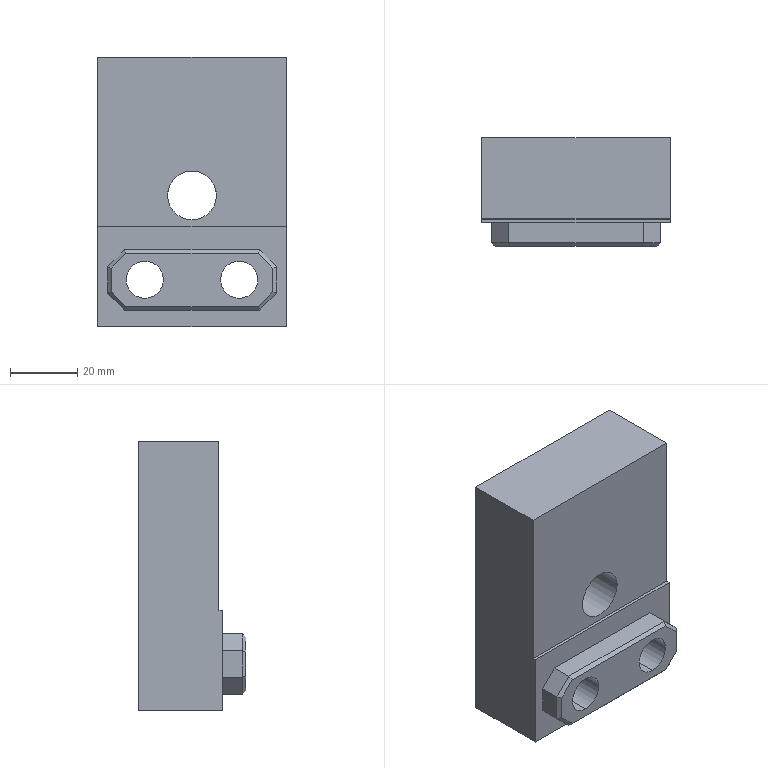Part | Creo | 1 solid | 53 faces | box 56 x 32 x 80 mm | volume 99961 mm3 | plane 27 | cylinder 18 | cone 8 | commonest cylinder face diameters 6.71 x4 8 x4 11 x4 18 x4 14.5 x2
STEP:
#1=CARTESIAN_POINT('',(0.,0.,0.));
#2=DIRECTION('',(0.,0.,1.));
#3=DIRECTION('',(1.,0.,0.));
#4=AXIS2_PLACEMENT_3D('',#1,#2,#3);
#5=CARTESIAN_POINT('',(-28.05,250.,-50.133));
#6=VERTEX_POINT('',#5);
#7=CARTESIAN_POINT('',(-28.05,250.,-20.267));
#8=VERTEX_POINT('',#7);
#9=CARTESIAN_POINT('',(-28.05,250.,-50.133));
#10=DIRECTION('',(0.,0.,1.));
#11=VECTOR('',#10,29.866);
#12=LINE('',#9,#11);
#13=EDGE_CURVE('',#6,#8,#12,.T.);
#14=ORIENTED_EDGE('',*,*,#13,.T.);
#15=CARTESIAN_POINT('',(27.95,250.,-20.267));
#16=VERTEX_POINT('',#15);
#17=CARTESIAN_POINT('',(27.95,250.,-20.267));
#18=DIRECTION('',(-1.,0.,0.));
#19=VECTOR('',#18,56.);
#20=LINE('',#17,#19);
#21=EDGE_CURVE('',#16,#8,#20,.T.);
#22=ORIENTED_EDGE('',*,*,#21,.F.);
#23=CARTESIAN_POINT('',(27.95,250.,-50.133));
#24=VERTEX_POINT('',#23);
#25=CARTESIAN_POINT('',(27.95,250.,-20.267));
#26=DIRECTION('',(0.,0.,-1.));
#27=VECTOR('',#26,29.866);
#28=LINE('',#25,#27);
#29=EDGE_CURVE('',#16,#24,#28,.T.);
#30=ORIENTED_EDGE('',*,*,#29,.T.);
#31=CARTESIAN_POINT('',(27.95,250.,-50.133));
#32=DIRECTION('',(-1.,0.,0.));
#33=VECTOR('',#32,56.);
#34=LINE('',#31,#33);
#35=EDGE_CURVE('',#24,#6,#34,.T.);
#36=ORIENTED_EDGE('',*,*,#35,.T.);
#37=EDGE_LOOP('',(#14,#22,#30,#36));
#38=FACE_OUTER_BOUND('',#37,.F.);
#39=CARTESIAN_POINT('',(-25.05,250.,-40.133));
#40=VERTEX_POINT('',#39);
#41=CARTESIAN_POINT('',(-25.05,250.,-32.267));
#42=VERTEX_POINT('',#41);
#43=CARTESIAN_POINT('',(-25.05,250.,-40.133));
#44=DIRECTION('',(0.,0.,1.));
#45=VECTOR('',#44,7.867);
#46=LINE('',#43,#45);
#47=EDGE_CURVE('',#40,#42,#46,.T.);
#48=ORIENTED_EDGE('',*,*,#47,.F.);
#49=CARTESIAN_POINT('',(-20.05,250.,-45.133));
#50=VERTEX_POINT('',#49);
#51=CARTESIAN_POINT('',(-20.05,250.,-45.133));
#52=DIRECTION('',(-0.7071,0.,0.7071));
#53=VECTOR('',#52,7.071);
#54=LINE('',#51,#53);
#55=EDGE_CURVE('',#50,#40,#54,.T.);
#56=ORIENTED_EDGE('',*,*,#55,.F.);
#57=CARTESIAN_POINT('',(19.95,250.,-45.133));
#58=VERTEX_POINT('',#57);
#59=CARTESIAN_POINT('',(-20.05,250.,-45.133));
#60=DIRECTION('',(1.,0.,0.));
#61=VECTOR('',#60,40.);
#62=LINE('',#59,#61);
#63=EDGE_CURVE('',#50,#58,#62,.T.);
#64=ORIENTED_EDGE('',*,*,#63,.T.);
#65=CARTESIAN_POINT('',(24.95,250.,-40.133));
#66=VERTEX_POINT('',#65);
#67=CARTESIAN_POINT('',(24.95,250.,-40.133));
#68=DIRECTION('',(-0.7071,0.,-0.7071));
#69=VECTOR('',#68,7.071);
#70=LINE('',#67,#69);
#71=EDGE_CURVE('',#66,#58,#70,.T.);
#72=ORIENTED_EDGE('',*,*,#71,.F.);
#73=CARTESIAN_POINT('',(24.95,250.,-32.267));
#74=VERTEX_POINT('',#73);
#75=CARTESIAN_POINT('',(24.95,250.,-32.267));
#76=DIRECTION('',(0.,0.,-1.));
#77=VECTOR('',#76,7.867);
#78=LINE('',#75,#77);
#79=EDGE_CURVE('',#74,#66,#78,.T.);
#80=ORIENTED_EDGE('',*,*,#79,.F.);
#81=CARTESIAN_POINT('',(19.95,250.,-27.267));
#82=VERTEX_POINT('',#81);
#83=CARTESIAN_POINT('',(19.95,250.,-27.267));
#84=DIRECTION('',(0.7071,0.,-0.7071));
#85=VECTOR('',#84,7.071);
#86=LINE('',#83,#85);
#87=EDGE_CURVE('',#82,#74,#86,.T.);
#88=ORIENTED_EDGE('',*,*,#87,.F.);
#89=CARTESIAN_POINT('',(-20.05,250.,-27.267));
#90=VERTEX_POINT('',#89);
#91=CARTESIAN_POINT('',(19.95,250.,-27.267));
#92=DIRECTION('',(-1.,0.,0.));
#93=VECTOR('',#92,40.);
#94=LINE('',#91,#93);
#95=EDGE_CURVE('',#82,#90,#94,.T.);
#96=ORIENTED_EDGE('',*,*,#95,.T.);
#97=CARTESIAN_POINT('',(-25.05,250.,-32.267));
#98=DIRECTION('',(0.7071,0.,0.7071));
#99=VECTOR('',#98,7.071);
#100=LINE('',#97,#99);
#101=EDGE_CURVE('',#42,#90,#100,.T.);
#102=ORIENTED_EDGE('',*,*,#101,.F.);
#103=EDGE_LOOP('',(#48,#56,#64,#72,#80,#88,#96,#102));
#104=FACE_BOUND('',#103,.F.);
#105=CARTESIAN_POINT('',(0.,250.,0.));
#106=DIRECTION('',(0.,-1.,0.));
#107=DIRECTION('',(0.,0.,-1.));
#108=AXIS2_PLACEMENT_3D('',#105,#106,#107);
#109=PLANE('',#108);
#110=ADVANCED_FACE('',(#38,#104),#109,.T.);
#111=CARTESIAN_POINT('',(-28.05,275.,-50.133));
#112=VERTEX_POINT('',#111);
#113=CARTESIAN_POINT('',(-28.05,275.,-50.133));
#114=DIRECTION('',(0.,-1.,0.));
#115=VECTOR('',#114,25.);
#116=LINE('',#113,#115);
#117=EDGE_CURVE('',#112,#6,#116,.T.);
#118=ORIENTED_EDGE('',*,*,#117,.F.);
#119=CARTESIAN_POINT('',(-28.05,275.,29.866));
#120=VERTEX_POINT('',#119);
#121=CARTESIAN_POINT('',(-28.05,275.,-50.133));
#122=DIRECTION('',(0.,0.,1.));
#123=VECTOR('',#122,80.);
#124=LINE('',#121,#123);
#125=EDGE_CURVE('',#112,#120,#124,.T.);
#126=ORIENTED_EDGE('',*,*,#125,.T.);
#127=CARTESIAN_POINT('',(-28.05,251.,29.866));
#128=VERTEX_POINT('',#127);
#129=CARTESIAN_POINT('',(-28.05,275.,29.866));
#130=DIRECTION('',(0.,-1.,0.));
#131=VECTOR('',#130,24.);
#132=LINE('',#129,#131);
#133=EDGE_CURVE('',#120,#128,#132,.T.);
#134=ORIENTED_EDGE('',*,*,#133,.T.);
#135=CARTESIAN_POINT('',(-28.05,251.,-20.267));
#136=VERTEX_POINT('',#135);
#137=CARTESIAN_POINT('',(-28.05,251.,-20.267));
#138=DIRECTION('',(0.,0.,1.));
#139=VECTOR('',#138,50.133);
#140=LINE('',#137,#139);
#141=EDGE_CURVE('',#136,#128,#140,.T.);
#142=ORIENTED_EDGE('',*,*,#141,.F.);
#143=CARTESIAN_POINT('',(-28.05,250.,-20.267));
#144=DIRECTION('',(0.,1.,0.));
#145=VECTOR('',#144,1.);
#146=LINE('',#143,#145);
#147=EDGE_CURVE('',#8,#136,#146,.T.);
#148=ORIENTED_EDGE('',*,*,#147,.F.);
#149=ORIENTED_EDGE('',*,*,#13,.F.);
#150=EDGE_LOOP('',(#118,#126,#134,#142,#148,#149));
#151=FACE_OUTER_BOUND('',#150,.F.);
#152=CARTESIAN_POINT('',(-28.05,250.,4.867));
#153=DIRECTION('',(1.,0.,0.));
#154=DIRECTION('',(0.,0.,-1.));
#155=AXIS2_PLACEMENT_3D('',#152,#153,#154);
#156=PLANE('',#155);
#157=ADVANCED_FACE('',(#151),#156,.F.);
#158=CARTESIAN_POINT('',(27.95,275.,-50.133));
#159=VERTEX_POINT('',#158);
#160=CARTESIAN_POINT('',(27.95,275.,-50.133));
#161=DIRECTION('',(-1.,0.,0.));
#162=VECTOR('',#161,56.);
#163=LINE('',#160,#162);
#164=EDGE_CURVE('',#159,#112,#163,.T.);
#165=ORIENTED_EDGE('',*,*,#164,.T.);
#166=ORIENTED_EDGE('',*,*,#117,.T.);
#167=ORIENTED_EDGE('',*,*,#35,.F.);
#168=CARTESIAN_POINT('',(27.95,275.,-50.133));
#169=DIRECTION('',(0.,-1.,0.));
#170=VECTOR('',#169,25.);
#171=LINE('',#168,#170);
#172=EDGE_CURVE('',#159,#24,#171,.T.);
#173=ORIENTED_EDGE('',*,*,#172,.F.);
#174=EDGE_LOOP('',(#165,#166,#167,#173));
#175=FACE_OUTER_BOUND('',#174,.F.);
#176=CARTESIAN_POINT('',(-25.05,250.,-50.133));
#177=DIRECTION('',(0.,0.,1.));
#178=DIRECTION('',(1.,0.,0.));
#179=AXIS2_PLACEMENT_3D('',#176,#177,#178);
#180=PLANE('',#179);
#181=ADVANCED_FACE('',(#175),#180,.F.);
#182=CARTESIAN_POINT('',(27.95,275.,29.866));
#183=VERTEX_POINT('',#182);
#184=CARTESIAN_POINT('',(27.95,275.,29.866));
#185=DIRECTION('',(0.,0.,-1.));
#186=VECTOR('',#185,80.);
#187=LINE('',#184,#186);
#188=EDGE_CURVE('',#183,#159,#187,.T.);
#189=ORIENTED_EDGE('',*,*,#188,.F.);
#190=CARTESIAN_POINT('',(-28.05,275.,29.866));
#191=DIRECTION('',(1.,0.,0.));
#192=VECTOR('',#191,56.);
#193=LINE('',#190,#192);
#194=EDGE_CURVE('',#120,#183,#193,.T.);
#195=ORIENTED_EDGE('',*,*,#194,.F.);
#196=ORIENTED_EDGE('',*,*,#125,.F.);
#197=ORIENTED_EDGE('',*,*,#164,.F.);
#198=EDGE_LOOP('',(#189,#195,#196,#197));
#199=FACE_OUTER_BOUND('',#198,.F.);
#200=CARTESIAN_POINT('',(-0.05,275.,-18.384));
#201=VERTEX_POINT('',#200);
#202=CARTESIAN_POINT('',(7.2,275.,-11.133));
#203=VERTEX_POINT('',#202);
#204=CARTESIAN_POINT('',(-0.05,275.,-11.133));
#205=DIRECTION('',(0.,-1.,0.));
#206=DIRECTION('',(0.,0.,-1.));
#207=AXIS2_PLACEMENT_3D('',#204,#205,#206);
#208=CIRCLE('',#207,7.25);
#209=EDGE_CURVE('',#201,#203,#208,.T.);
#210=ORIENTED_EDGE('',*,*,#209,.F.);
#211=CARTESIAN_POINT('',(-7.3,275.,-11.133));
#212=VERTEX_POINT('',#211);
#213=CARTESIAN_POINT('',(-0.05,275.,-11.133));
#214=DIRECTION('',(0.,-1.,0.));
#215=DIRECTION('',(-1.,0.,0.));
#216=AXIS2_PLACEMENT_3D('',#213,#214,#215);
#217=CIRCLE('',#216,7.25);
#218=EDGE_CURVE('',#212,#201,#217,.T.);
#219=ORIENTED_EDGE('',*,*,#218,.F.);
#220=CARTESIAN_POINT('',(-0.05,275.,-3.884));
#221=VERTEX_POINT('',#220);
#222=CARTESIAN_POINT('',(-0.05,275.,-11.133));
#223=DIRECTION('',(0.,-1.,0.));
#224=DIRECTION('',(0.,0.,1.));
#225=AXIS2_PLACEMENT_3D('',#222,#223,#224);
#226=CIRCLE('',#225,7.25);
#227=EDGE_CURVE('',#221,#212,#226,.T.);
#228=ORIENTED_EDGE('',*,*,#227,.F.);
#229=CARTESIAN_POINT('',(-0.05,275.,-11.133));
#230=DIRECTION('',(0.,-1.,0.));
#231=DIRECTION('',(1.,0.,0.));
#232=AXIS2_PLACEMENT_3D('',#229,#230,#231);
#233=CIRCLE('',#232,7.25);
#234=EDGE_CURVE('',#203,#221,#233,.T.);
#235=ORIENTED_EDGE('',*,*,#234,.F.);
#236=EDGE_LOOP('',(#210,#219,#228,#235));
#237=FACE_BOUND('',#236,.F.);
#238=CARTESIAN_POINT('',(13.95,275.,-45.133));
#239=VERTEX_POINT('',#238);
#240=CARTESIAN_POINT('',(13.95,275.,-27.134));
#241=VERTEX_POINT('',#240);
#242=CARTESIAN_POINT('',(13.95,275.,-36.133));
#243=DIRECTION('',(0.,-1.,0.));
#244=DIRECTION('',(0.,0.,-1.));
#245=AXIS2_PLACEMENT_3D('',#242,#243,#244);
#246=CIRCLE('',#245,9.);
#247=EDGE_CURVE('',#239,#241,#246,.T.);
#248=ORIENTED_EDGE('',*,*,#247,.F.);
#249=CARTESIAN_POINT('',(13.95,275.,-36.133));
#250=DIRECTION('',(0.,-1.,0.));
#251=DIRECTION('',(0.,0.,1.));
#252=AXIS2_PLACEMENT_3D('',#249,#250,#251);
#253=CIRCLE('',#252,9.);
#254=EDGE_CURVE('',#241,#239,#253,.T.);
#255=ORIENTED_EDGE('',*,*,#254,.F.);
#256=EDGE_LOOP('',(#248,#255));
#257=FACE_BOUND('',#256,.F.);
#258=CARTESIAN_POINT('',(-14.05,275.,-45.133));
#259=VERTEX_POINT('',#258);
#260=CARTESIAN_POINT('',(-14.05,275.,-27.134));
#261=VERTEX_POINT('',#260);
#262=CARTESIAN_POINT('',(-14.05,275.,-36.133));
#263=DIRECTION('',(0.,-1.,0.));
#264=DIRECTION('',(0.,0.,-1.));
#265=AXIS2_PLACEMENT_3D('',#262,#263,#264);
#266=CIRCLE('',#265,9.);
#267=EDGE_CURVE('',#259,#261,#266,.T.);
#268=ORIENTED_EDGE('',*,*,#267,.F.);
#269=CARTESIAN_POINT('',(-14.05,275.,-36.133));
#270=DIRECTION('',(0.,-1.,0.));
#271=DIRECTION('',(0.,0.,1.));
#272=AXIS2_PLACEMENT_3D('',#269,#270,#271);
#273=CIRCLE('',#272,9.);
#274=EDGE_CURVE('',#261,#259,#273,.T.);
#275=ORIENTED_EDGE('',*,*,#274,.F.);
#276=EDGE_LOOP('',(#268,#275));
#277=FACE_BOUND('',#276,.F.);
#278=CARTESIAN_POINT('',(15.95,275.,18.42));
#279=VERTEX_POINT('',#278);
#280=CARTESIAN_POINT('',(7.95,275.,18.42));
#281=VERTEX_POINT('',#280);
#282=CARTESIAN_POINT('',(11.95,275.,18.42));
#283=DIRECTION('',(0.,-1.,0.));
#284=DIRECTION('',(1.,0.,0.));
#285=AXIS2_PLACEMENT_3D('',#282,#283,#284);
#286=CIRCLE('',#285,4.);
#287=EDGE_CURVE('',#279,#281,#286,.T.);
#288=ORIENTED_EDGE('',*,*,#287,.F.);
#289=CARTESIAN_POINT('',(11.95,275.,18.42));
#290=DIRECTION('',(0.,-1.,0.));
#291=DIRECTION('',(-1.,0.,0.));
#292=AXIS2_PLACEMENT_3D('',#289,#290,#291);
#293=CIRCLE('',#292,4.);
#294=EDGE_CURVE('',#281,#279,#293,.T.);
#295=ORIENTED_EDGE('',*,*,#294,.F.);
#296=EDGE_LOOP('',(#288,#295));
#297=FACE_BOUND('',#296,.F.);
#298=CARTESIAN_POINT('',(-8.05,275.,18.42));
#299=VERTEX_POINT('',#298);
#300=CARTESIAN_POINT('',(-16.05,275.,18.42));
#301=VERTEX_POINT('',#300);
#302=CARTESIAN_POINT('',(-12.05,275.,18.42));
#303=DIRECTION('',(0.,-1.,0.));
#304=DIRECTION('',(1.,0.,0.));
#305=AXIS2_PLACEMENT_3D('',#302,#303,#304);
#306=CIRCLE('',#305,4.);
#307=EDGE_CURVE('',#299,#301,#306,.T.);
#308=ORIENTED_EDGE('',*,*,#307,.F.);
#309=CARTESIAN_POINT('',(-12.05,275.,18.42));
#310=DIRECTION('',(0.,-1.,0.));
#311=DIRECTION('',(-1.,0.,0.));
#312=AXIS2_PLACEMENT_3D('',#309,#310,#311);
#313=CIRCLE('',#312,4.);
#314=EDGE_CURVE('',#301,#299,#313,.T.);
#315=ORIENTED_EDGE('',*,*,#314,.F.);
#316=EDGE_LOOP('',(#308,#315));
#317=FACE_BOUND('',#316,.F.);
#318=CARTESIAN_POINT('',(0.,275.,0.));
#319=DIRECTION('',(0.,-1.,0.));
#320=DIRECTION('',(0.,0.,-1.));
#321=AXIS2_PLACEMENT_3D('',#318,#319,#320);
#322=PLANE('',#321);
#323=ADVANCED_FACE('',(#199,#237,#257,#277,#297,#317),#322,.F.);
#324=CARTESIAN_POINT('',(7.2,251.,-11.133));
#325=VERTEX_POINT('',#324);
#326=CARTESIAN_POINT('',(-0.05,251.,-18.384));
#327=VERTEX_POINT('',#326);
#328=CARTESIAN_POINT('',(-0.05,251.,-11.133));
#329=DIRECTION('',(0.,1.,0.));
#330=DIRECTION('',(1.,0.,0.));
#331=AXIS2_PLACEMENT_3D('',#328,#329,#330);
#332=CIRCLE('',#331,7.25);
#333=EDGE_CURVE('',#325,#327,#332,.T.);
#334=ORIENTED_EDGE('',*,*,#333,.T.);
#335=CARTESIAN_POINT('',(-7.3,251.,-11.133));
#336=VERTEX_POINT('',#335);
#337=CARTESIAN_POINT('',(-0.05,251.,-11.133));
#338=DIRECTION('',(0.,1.,0.));
#339=DIRECTION('',(0.,0.,-1.));
#340=AXIS2_PLACEMENT_3D('',#337,#338,#339);
#341=CIRCLE('',#340,7.25);
#342=EDGE_CURVE('',#327,#336,#341,.T.);
#343=ORIENTED_EDGE('',*,*,#342,.T.);
#344=CARTESIAN_POINT('',(-7.3,251.,-11.133));
#345=DIRECTION('',(0.,1.,0.));
#346=VECTOR('',#345,24.);
#347=LINE('',#344,#346);
#348=EDGE_CURVE('',#336,#212,#347,.T.);
#349=ORIENTED_EDGE('',*,*,#348,.T.);
#350=ORIENTED_EDGE('',*,*,#218,.T.);
#351=ORIENTED_EDGE('',*,*,#209,.T.);
#352=CARTESIAN_POINT('',(7.2,251.,-11.133));
#353=DIRECTION('',(0.,1.,0.));
#354=VECTOR('',#353,24.);
#355=LINE('',#352,#354);
#356=EDGE_CURVE('',#325,#203,#355,.T.);
#357=ORIENTED_EDGE('',*,*,#356,.F.);
#358=EDGE_LOOP('',(#334,#343,#349,#350,#351,#357));
#359=FACE_OUTER_BOUND('',#358,.F.);
#360=CARTESIAN_POINT('',(-0.05,205.,-11.133));
#361=DIRECTION('',(0.,1.,0.));
#362=DIRECTION('',(-1.,0.,0.));
#363=AXIS2_PLACEMENT_3D('',#360,#361,#362);
#364=CYLINDRICAL_SURFACE('',#363,7.25);
#365=ADVANCED_FACE('',(#359),#364,.F.);
#366=ORIENTED_EDGE('',*,*,#141,.T.);
#367=CARTESIAN_POINT('',(27.95,251.,29.866));
#368=VERTEX_POINT('',#367);
#369=CARTESIAN_POINT('',(-28.05,251.,29.866));
#370=DIRECTION('',(1.,0.,0.));
#371=VECTOR('',#370,56.);
#372=LINE('',#369,#371);
#373=EDGE_CURVE('',#128,#368,#372,.T.);
#374=ORIENTED_EDGE('',*,*,#373,.T.);
#375=CARTESIAN_POINT('',(27.95,251.,-20.267));
#376=VERTEX_POINT('',#375);
#377=CARTESIAN_POINT('',(27.95,251.,29.866));
#378=DIRECTION('',(0.,0.,-1.));
#379=VECTOR('',#378,50.133);
#380=LINE('',#377,#379);
#381=EDGE_CURVE('',#368,#376,#380,.T.);
#382=ORIENTED_EDGE('',*,*,#381,.T.);
#383=CARTESIAN_POINT('',(-28.05,251.,-20.267));
#384=DIRECTION('',(1.,0.,0.));
#385=VECTOR('',#384,56.);
#386=LINE('',#383,#385);
#387=EDGE_CURVE('',#136,#376,#386,.T.);
#388=ORIENTED_EDGE('',*,*,#387,.F.);
#389=EDGE_LOOP('',(#366,#374,#382,#388));
#390=FACE_OUTER_BOUND('',#389,.F.);
#391=ORIENTED_EDGE('',*,*,#342,.F.);
#392=ORIENTED_EDGE('',*,*,#333,.F.);
#393=CARTESIAN_POINT('',(-0.05,251.,-11.133));
#394=DIRECTION('',(0.,1.,0.));
#395=DIRECTION('',(-1.,0.,0.));
#396=AXIS2_PLACEMENT_3D('',#393,#394,#395);
#397=CIRCLE('',#396,7.25);
#398=EDGE_CURVE('',#336,#325,#397,.T.);
#399=ORIENTED_EDGE('',*,*,#398,.F.);
#400=EDGE_LOOP('',(#391,#392,#399));
#401=FACE_BOUND('',#400,.F.);
#402=CARTESIAN_POINT('',(0.,251.,0.));
#403=DIRECTION('',(0.,-1.,0.));
#404=DIRECTION('',(0.,0.,-1.));
#405=AXIS2_PLACEMENT_3D('',#402,#403,#404);
#406=PLANE('',#405);
#407=ADVANCED_FACE('',(#390,#401),#406,.T.);
#408=ORIENTED_EDGE('',*,*,#398,.T.);
#409=ORIENTED_EDGE('',*,*,#356,.T.);
#410=ORIENTED_EDGE('',*,*,#234,.T.);
#411=ORIENTED_EDGE('',*,*,#227,.T.);
#412=ORIENTED_EDGE('',*,*,#348,.F.);
#413=EDGE_LOOP('',(#408,#409,#410,#411,#412));
#414=FACE_OUTER_BOUND('',#413,.F.);
#415=CARTESIAN_POINT('',(-0.05,205.,-11.133));
#416=DIRECTION('',(0.,1.,0.));
#417=DIRECTION('',(-1.,0.,0.));
#418=AXIS2_PLACEMENT_3D('',#415,#416,#417);
#419=CYLINDRICAL_SURFACE('',#418,7.25);
#420=ADVANCED_FACE('',(#414),#419,.F.);
#421=ORIENTED_EDGE('',*,*,#194,.T.);
#422=CARTESIAN_POINT('',(27.95,275.,29.866));
#423=DIRECTION('',(0.,-1.,0.));
#424=VECTOR('',#423,24.);
#425=LINE('',#422,#424);
#426=EDGE_CURVE('',#183,#368,#425,.T.);
#427=ORIENTED_EDGE('',*,*,#426,.T.);
#428=ORIENTED_EDGE('',*,*,#373,.F.);
#429=ORIENTED_EDGE('',*,*,#133,.F.);
#430=EDGE_LOOP('',(#421,#427,#428,#429));
#431=FACE_OUTER_BOUND('',#430,.F.);
#432=CARTESIAN_POINT('',(24.95,250.,29.866));
#433=DIRECTION('',(0.,0.,-1.));
#434=DIRECTION('',(-1.,0.,0.));
#435=AXIS2_PLACEMENT_3D('',#432,#433,#434);
#436=PLANE('',#435);
#437=ADVANCED_FACE('',(#431),#436,.F.);
#438=ORIENTED_EDGE('',*,*,#29,.F.);
#439=CARTESIAN_POINT('',(27.95,251.,-20.267));
#440=DIRECTION('',(0.,-1.,0.));
#441=VECTOR('',#440,1.);
#442=LINE('',#439,#441);
#443=EDGE_CURVE('',#376,#16,#442,.T.);
#444=ORIENTED_EDGE('',*,*,#443,.F.);
#445=ORIENTED_EDGE('',*,*,#381,.F.);
#446=ORIENTED_EDGE('',*,*,#426,.F.);
#447=ORIENTED_EDGE('',*,*,#188,.T.);
#448=ORIENTED_EDGE('',*,*,#172,.T.);
#449=EDGE_LOOP('',(#438,#444,#445,#446,#447,#448));
#450=FACE_OUTER_BOUND('',#449,.F.);
#451=CARTESIAN_POINT('',(27.95,250.,-50.133));
#452=DIRECTION('',(-1.,0.,0.));
#453=DIRECTION('',(0.,0.,1.));
#454=AXIS2_PLACEMENT_3D('',#451,#452,#453);
#455=PLANE('',#454);
#456=ADVANCED_FACE('',(#450),#455,.F.);
#457=ORIENTED_EDGE('',*,*,#443,.T.);
#458=ORIENTED_EDGE('',*,*,#21,.T.);
#459=ORIENTED_EDGE('',*,*,#147,.T.);
#460=ORIENTED_EDGE('',*,*,#387,.T.);
#461=EDGE_LOOP('',(#457,#458,#459,#460));
#462=FACE_OUTER_BOUND('',#461,.F.);
#463=CARTESIAN_POINT('',(-0.05,205.5,-20.267));
#464=DIRECTION('',(0.,0.,-1.));
#465=DIRECTION('',(-1.,0.,0.));
#466=AXIS2_PLACEMENT_3D('',#463,#464,#465);
#467=PLANE('',#466);
#468=ADVANCED_FACE('',(#462),#467,.F.);
#469=CARTESIAN_POINT('',(13.95,264.,-27.134));
#470=VERTEX_POINT('',#469);
#471=CARTESIAN_POINT('',(13.95,264.,-45.133));
#472=VERTEX_POINT('',#471);
#473=CARTESIAN_POINT('',(13.95,264.,-36.133));
#474=DIRECTION('',(0.,1.,0.));
#475=DIRECTION('',(0.,0.,1.));
#476=AXIS2_PLACEMENT_3D('',#473,#474,#475);
#477=CIRCLE('',#476,9.);
#478=EDGE_CURVE('',#470,#472,#477,.T.);
#479=ORIENTED_EDGE('',*,*,#478,.T.);
#480=CARTESIAN_POINT('',(13.95,275.,-45.133));
#481=DIRECTION('',(0.,-1.,0.));
#482=VECTOR('',#481,11.);
#483=LINE('',#480,#482);
#484=EDGE_CURVE('',#239,#472,#483,.T.);
#485=ORIENTED_EDGE('',*,*,#484,.F.);
#486=ORIENTED_EDGE('',*,*,#247,.T.);
#487=CARTESIAN_POINT('',(13.95,275.,-27.134));
#488=DIRECTION('',(0.,-1.,0.));
#489=VECTOR('',#488,11.);
#490=LINE('',#487,#489);
#491=EDGE_CURVE('',#241,#470,#490,.T.);
#492=ORIENTED_EDGE('',*,*,#491,.T.);
#493=EDGE_LOOP('',(#479,#485,#486,#492));
#494=FACE_OUTER_BOUND('',#493,.F.);
#495=CARTESIAN_POINT('',(13.95,275.,-36.133));
#496=DIRECTION('',(0.,-1.,0.));
#497=DIRECTION('',(0.,0.,-1.));
#498=AXIS2_PLACEMENT_3D('',#495,#496,#497);
#499=CYLINDRICAL_SURFACE('',#498,9.);
#500=ADVANCED_FACE('',(#494),#499,.F.);
#501=CARTESIAN_POINT('',(13.95,264.,-36.133));
#502=DIRECTION('',(0.,1.,0.));
#503=DIRECTION('',(0.,0.,-1.));
#504=AXIS2_PLACEMENT_3D('',#501,#502,#503);
#505=CIRCLE('',#504,9.);
#506=EDGE_CURVE('',#472,#470,#505,.T.);
#507=ORIENTED_EDGE('',*,*,#506,.F.);
#508=ORIENTED_EDGE('',*,*,#478,.F.);
#509=EDGE_LOOP('',(#507,#508));
#510=FACE_OUTER_BOUND('',#509,.F.);
#511=CARTESIAN_POINT('',(13.95,264.,-41.633));
#512=VERTEX_POINT('',#511);
#513=CARTESIAN_POINT('',(13.95,264.,-30.634));
#514=VERTEX_POINT('',#513);
#515=CARTESIAN_POINT('',(13.95,264.,-36.133));
#516=DIRECTION('',(0.,-1.,0.));
#517=DIRECTION('',(0.,0.,-1.));
#518=AXIS2_PLACEMENT_3D('',#515,#516,#517);
#519=CIRCLE('',#518,5.5);
#520=EDGE_CURVE('',#512,#514,#519,.T.);
#521=ORIENTED_EDGE('',*,*,#520,.F.);
#522=CARTESIAN_POINT('',(13.95,264.,-36.133));
#523=DIRECTION('',(0.,-1.,0.));
#524=DIRECTION('',(0.,0.,1.));
#525=AXIS2_PLACEMENT_3D('',#522,#523,#524);
#526=CIRCLE('',#525,5.5);
#527=EDGE_CURVE('',#514,#512,#526,.T.);
#528=ORIENTED_EDGE('',*,*,#527,.F.);
#529=EDGE_LOOP('',(#521,#528));
#530=FACE_BOUND('',#529,.F.);
#531=CARTESIAN_POINT('',(13.95,264.,-36.133));
#532=DIRECTION('',(0.,-1.,0.));
#533=DIRECTION('',(0.,0.,-1.));
#534=AXIS2_PLACEMENT_3D('',#531,#532,#533);
#535=PLANE('',#534);
#536=ADVANCED_FACE('',(#510,#530),#535,.F.);
#537=ORIENTED_EDGE('',*,*,#520,.T.);
#538=CARTESIAN_POINT('',(13.95,243.,-30.634));
#539=VERTEX_POINT('',#538);
#540=CARTESIAN_POINT('',(13.95,264.,-30.634));
#541=DIRECTION('',(0.,-1.,0.));
#542=VECTOR('',#541,21.);
#543=LINE('',#540,#542);
#544=EDGE_CURVE('',#514,#539,#543,.T.);
#545=ORIENTED_EDGE('',*,*,#544,.T.);
#546=CARTESIAN_POINT('',(13.95,243.,-41.633));
#547=VERTEX_POINT('',#546);
#548=CARTESIAN_POINT('',(13.95,243.,-36.133));
#549=DIRECTION('',(0.,1.,0.));
#550=DIRECTION('',(0.,0.,1.));
#551=AXIS2_PLACEMENT_3D('',#548,#549,#550);
#552=CIRCLE('',#551,5.5);
#553=EDGE_CURVE('',#539,#547,#552,.T.);
#554=ORIENTED_EDGE('',*,*,#553,.T.);
#555=CARTESIAN_POINT('',(13.95,264.,-41.633));
#556=DIRECTION('',(0.,-1.,0.));
#557=VECTOR('',#556,21.);
#558=LINE('',#555,#557);
#559=EDGE_CURVE('',#512,#547,#558,.T.);
#560=ORIENTED_EDGE('',*,*,#559,.F.);
#561=EDGE_LOOP('',(#537,#545,#554,#560));
#562=FACE_OUTER_BOUND('',#561,.F.);
#563=CARTESIAN_POINT('',(13.95,75.,-36.133));
#564=DIRECTION('',(0.,-1.,0.));
#565=DIRECTION('',(0.,0.,-1.));
#566=AXIS2_PLACEMENT_3D('',#563,#564,#565);
#567=CYLINDRICAL_SURFACE('',#566,5.5);
#568=ADVANCED_FACE('',(#562),#567,.F.);
#569=ORIENTED_EDGE('',*,*,#527,.T.);
#570=ORIENTED_EDGE('',*,*,#559,.T.);
#571=CARTESIAN_POINT('',(13.95,243.,-36.133));
#572=DIRECTION('',(0.,1.,0.));
#573=DIRECTION('',(0.,0.,-1.));
#574=AXIS2_PLACEMENT_3D('',#571,#572,#573);
#575=CIRCLE('',#574,5.5);
#576=EDGE_CURVE('',#547,#539,#575,.T.);
#577=ORIENTED_EDGE('',*,*,#576,.T.);
#578=ORIENTED_EDGE('',*,*,#544,.F.);
#579=EDGE_LOOP('',(#569,#570,#577,#578));
#580=FACE_OUTER_BOUND('',#579,.F.);
#581=CARTESIAN_POINT('',(13.95,75.,-36.133));
#582=DIRECTION('',(0.,-1.,0.));
#583=DIRECTION('',(0.,0.,-1.));
#584=AXIS2_PLACEMENT_3D('',#581,#582,#583);
#585=CYLINDRICAL_SURFACE('',#584,5.5);
#586=ADVANCED_FACE('',(#580),#585,.F.);
#587=CARTESIAN_POINT('',(23.95,243.,-32.681));
#588=VERTEX_POINT('',#587);
#589=CARTESIAN_POINT('',(23.95,243.,-39.719));
#590=VERTEX_POINT('',#589);
#591=CARTESIAN_POINT('',(23.95,243.,-32.681));
#592=DIRECTION('',(0.,0.,-1.));
#593=VECTOR('',#592,7.038);
#594=LINE('',#591,#593);
#595=EDGE_CURVE('',#588,#590,#594,.T.);
#596=ORIENTED_EDGE('',*,*,#595,.T.);
#597=CARTESIAN_POINT('',(19.536,243.,-44.133));
#598=VERTEX_POINT('',#597);
#599=CARTESIAN_POINT('',(19.536,243.,-44.133));
#600=DIRECTION('',(0.7071,0.,0.7071));
#601=VECTOR('',#600,6.243);
#602=LINE('',#599,#601);
#603=EDGE_CURVE('',#598,#590,#602,.T.);
#604=ORIENTED_EDGE('',*,*,#603,.F.);
#605=CARTESIAN_POINT('',(-19.636,243.,-44.133));
#606=VERTEX_POINT('',#605);
#607=CARTESIAN_POINT('',(19.536,243.,-44.133));
#608=DIRECTION('',(-1.,0.,0.));
#609=VECTOR('',#608,39.172);
#610=LINE('',#607,#609);
#611=EDGE_CURVE('',#598,#606,#610,.T.);
#612=ORIENTED_EDGE('',*,*,#611,.T.);
#613=CARTESIAN_POINT('',(-24.05,243.,-39.719));
#614=VERTEX_POINT('',#613);
#615=CARTESIAN_POINT('',(-24.05,243.,-39.719));
#616=DIRECTION('',(0.7071,0.,-0.7071));
#617=VECTOR('',#616,6.243);
#618=LINE('',#615,#617);
#619=EDGE_CURVE('',#614,#606,#618,.T.);
#620=ORIENTED_EDGE('',*,*,#619,.F.);
#621=CARTESIAN_POINT('',(-24.05,243.,-32.681));
#622=VERTEX_POINT('',#621);
#623=CARTESIAN_POINT('',(-24.05,243.,-39.719));
#624=DIRECTION('',(0.,0.,1.));
#625=VECTOR('',#624,7.038);
#626=LINE('',#623,#625);
#627=EDGE_CURVE('',#614,#622,#626,.T.);
#628=ORIENTED_EDGE('',*,*,#627,.T.);
#629=CARTESIAN_POINT('',(-19.636,243.,-28.267));
#630=VERTEX_POINT('',#629);
#631=CARTESIAN_POINT('',(-19.636,243.,-28.267));
#632=DIRECTION('',(-0.7071,0.,-0.7071));
#633=VECTOR('',#632,6.243);
#634=LINE('',#631,#633);
#635=EDGE_CURVE('',#630,#622,#634,.T.);
#636=ORIENTED_EDGE('',*,*,#635,.F.);
#637=CARTESIAN_POINT('',(19.536,243.,-28.267));
#638=VERTEX_POINT('',#637);
#639=CARTESIAN_POINT('',(-19.636,243.,-28.267));
#640=DIRECTION('',(1.,0.,0.));
#641=VECTOR('',#640,39.172);
#642=LINE('',#639,#641);
#643=EDGE_CURVE('',#630,#638,#642,.T.);
#644=ORIENTED_EDGE('',*,*,#643,.T.);
#645=CARTESIAN_POINT('',(23.95,243.,-32.681));
#646=DIRECTION('',(-0.7071,0.,0.7071));
#647=VECTOR('',#646,6.243);
#648=LINE('',#645,#647);
#649=EDGE_CURVE('',#588,#638,#648,.T.);
#650=ORIENTED_EDGE('',*,*,#649,.F.);
#651=EDGE_LOOP('',(#596,#604,#612,#620,#628,#636,#644,#650));
#652=FACE_OUTER_BOUND('',#651,.F.);
#653=CARTESIAN_POINT('',(-14.05,243.,-41.633));
#654=VERTEX_POINT('',#653);
#655=CARTESIAN_POINT('',(-14.05,243.,-30.634));
#656=VERTEX_POINT('',#655);
#657=CARTESIAN_POINT('',(-14.05,243.,-36.133));
#658=DIRECTION('',(0.,1.,0.));
#659=DIRECTION('',(0.,0.,-1.));
#660=AXIS2_PLACEMENT_3D('',#657,#658,#659);
#661=CIRCLE('',#660,5.5);
#662=EDGE_CURVE('',#654,#656,#661,.T.);
#663=ORIENTED_EDGE('',*,*,#662,.F.);
#664=CARTESIAN_POINT('',(-14.05,243.,-36.133));
#665=DIRECTION('',(0.,1.,0.));
#666=DIRECTION('',(0.,0.,1.));
#667=AXIS2_PLACEMENT_3D('',#664,#665,#666);
#668=CIRCLE('',#667,5.5);
#669=EDGE_CURVE('',#656,#654,#668,.T.);
#670=ORIENTED_EDGE('',*,*,#669,.F.);
#671=EDGE_LOOP('',(#663,#670));
#672=FACE_BOUND('',#671,.F.);
#673=ORIENTED_EDGE('',*,*,#576,.F.);
#674=ORIENTED_EDGE('',*,*,#553,.F.);
#675=EDGE_LOOP('',(#673,#674));
#676=FACE_BOUND('',#675,.F.);
#677=CARTESIAN_POINT('',(-0.05,243.,-51.133));
#678=DIRECTION('',(0.,-1.,0.));
#679=DIRECTION('',(0.,0.,-1.));
#680=AXIS2_PLACEMENT_3D('',#677,#678,#679);
#681=PLANE('',#680);
#682=ADVANCED_FACE('',(#652,#672,#676),#681,.T.);
#683=CARTESIAN_POINT('',(24.95,244.,-40.133));
#684=VERTEX_POINT('',#683);
#685=CARTESIAN_POINT('',(24.95,244.,-40.133));
#686=DIRECTION('',(-0.6786,-0.6786,0.2811));
#687=VECTOR('',#686,1.474);
#688=LINE('',#685,#687);
#689=EDGE_CURVE('',#684,#590,#688,.T.);
#690=ORIENTED_EDGE('',*,*,#689,.T.);
#691=ORIENTED_EDGE('',*,*,#595,.F.);
#692=CARTESIAN_POINT('',(24.95,244.,-32.267));
#693=VERTEX_POINT('',#692);
#694=CARTESIAN_POINT('',(24.95,244.,-32.267));
#695=DIRECTION('',(-0.6786,-0.6786,-0.2811));
#696=VECTOR('',#695,1.474);
#697=LINE('',#694,#696);
#698=EDGE_CURVE('',#693,#588,#697,.T.);
#699=ORIENTED_EDGE('',*,*,#698,.F.);
#700=CARTESIAN_POINT('',(24.95,244.,-40.133));
#701=DIRECTION('',(0.,0.,1.));
#702=VECTOR('',#701,7.867);
#703=LINE('',#700,#702);
#704=EDGE_CURVE('',#684,#693,#703,.T.);
#705=ORIENTED_EDGE('',*,*,#704,.F.);
#706=EDGE_LOOP('',(#690,#691,#699,#705));
#707=FACE_OUTER_BOUND('',#706,.F.);
#708=CARTESIAN_POINT('',(23.95,243.,-51.133));
#709=DIRECTION('',(0.7071,-0.7071,0.));
#710=DIRECTION('',(0.,0.,-1.));
#711=AXIS2_PLACEMENT_3D('',#708,#709,#710);
#712=PLANE('',#711);
#713=ADVANCED_FACE('',(#707),#712,.T.);
#714=CARTESIAN_POINT('',(19.95,244.,-45.133));
#715=VERTEX_POINT('',#714);
#716=CARTESIAN_POINT('',(19.95,244.,-45.133));
#717=DIRECTION('',(-0.2811,-0.6786,0.6786));
#718=VECTOR('',#717,1.474);
#719=LINE('',#716,#718);
#720=EDGE_CURVE('',#715,#598,#719,.T.);
#721=ORIENTED_EDGE('',*,*,#720,.T.);
#722=ORIENTED_EDGE('',*,*,#603,.T.);
#723=ORIENTED_EDGE('',*,*,#689,.F.);
#724=CARTESIAN_POINT('',(19.95,244.,-45.133));
#725=DIRECTION('',(0.7071,0.,0.7071));
#726=VECTOR('',#725,7.071);
#727=LINE('',#724,#726);
#728=EDGE_CURVE('',#715,#684,#727,.T.);
#729=ORIENTED_EDGE('',*,*,#728,.F.);
#730=EDGE_LOOP('',(#721,#722,#723,#729));
#731=FACE_OUTER_BOUND('',#730,.F.);
#732=CARTESIAN_POINT('',(6.243,243.,-57.426));
#733=DIRECTION('',(0.5,-0.7071,-0.5));
#734=DIRECTION('',(-0.7071,0.,-0.7071));
#735=AXIS2_PLACEMENT_3D('',#732,#733,#734);
#736=PLANE('',#735);
#737=ADVANCED_FACE('',(#731),#736,.T.);
#738=CARTESIAN_POINT('',(-20.05,244.,-45.133));
#739=VERTEX_POINT('',#738);
#740=CARTESIAN_POINT('',(-20.05,244.,-45.133));
#741=DIRECTION('',(0.2811,-0.6786,0.6786));
#742=VECTOR('',#741,1.474);
#743=LINE('',#740,#742);
#744=EDGE_CURVE('',#739,#606,#743,.T.);
#745=ORIENTED_EDGE('',*,*,#744,.T.);
#746=ORIENTED_EDGE('',*,*,#611,.F.);
#747=ORIENTED_EDGE('',*,*,#720,.F.);
#748=CARTESIAN_POINT('',(-20.05,244.,-45.133));
#749=DIRECTION('',(1.,0.,0.));
#750=VECTOR('',#749,40.);
#751=LINE('',#748,#750);
#752=EDGE_CURVE('',#739,#715,#751,.T.);
#753=ORIENTED_EDGE('',*,*,#752,.F.);
#754=EDGE_LOOP('',(#745,#746,#747,#753));
#755=FACE_OUTER_BOUND('',#754,.F.);
#756=CARTESIAN_POINT('',(-0.05,243.,-44.133));
#757=DIRECTION('',(0.,-0.7071,-0.7071));
#758=DIRECTION('',(-1.,0.,0.));
#759=AXIS2_PLACEMENT_3D('',#756,#757,#758);
#760=PLANE('',#759);
#761=ADVANCED_FACE('',(#755),#760,.T.);
#762=CARTESIAN_POINT('',(-25.05,244.,-40.133));
#763=VERTEX_POINT('',#762);
#764=CARTESIAN_POINT('',(-24.05,243.,-39.719));
#765=DIRECTION('',(-0.6786,0.6786,-0.2811));
#766=VECTOR('',#765,1.474);
#767=LINE('',#764,#766);
#768=EDGE_CURVE('',#614,#763,#767,.T.);
#769=ORIENTED_EDGE('',*,*,#768,.F.);
#770=ORIENTED_EDGE('',*,*,#619,.T.);
#771=ORIENTED_EDGE('',*,*,#744,.F.);
#772=CARTESIAN_POINT('',(-25.05,244.,-40.133));
#773=DIRECTION('',(0.7071,0.,-0.7071));
#774=VECTOR('',#773,7.071);
#775=LINE('',#772,#774);
#776=EDGE_CURVE('',#763,#739,#775,.T.);
#777=ORIENTED_EDGE('',*,*,#776,.F.);
#778=EDGE_LOOP('',(#769,#770,#771,#777));
#779=FACE_OUTER_BOUND('',#778,.F.);
#780=CARTESIAN_POINT('',(-6.343,243.,-57.426));
#781=DIRECTION('',(-0.5,-0.7071,-0.5));
#782=DIRECTION('',(-0.7071,0.,0.7071));
#783=AXIS2_PLACEMENT_3D('',#780,#781,#782);
#784=PLANE('',#783);
#785=ADVANCED_FACE('',(#779),#784,.T.);
#786=ORIENTED_EDGE('',*,*,#768,.T.);
#787=CARTESIAN_POINT('',(-25.05,244.,-32.267));
#788=VERTEX_POINT('',#787);
#789=CARTESIAN_POINT('',(-25.05,244.,-32.267));
#790=DIRECTION('',(0.,0.,-1.));
#791=VECTOR('',#790,7.867);
#792=LINE('',#789,#791);
#793=EDGE_CURVE('',#788,#763,#792,.T.);
#794=ORIENTED_EDGE('',*,*,#793,.F.);
#795=CARTESIAN_POINT('',(-24.05,243.,-32.681));
#796=DIRECTION('',(-0.6786,0.6786,0.2811));
#797=VECTOR('',#796,1.474);
#798=LINE('',#795,#797);
#799=EDGE_CURVE('',#622,#788,#798,.T.);
#800=ORIENTED_EDGE('',*,*,#799,.F.);
#801=ORIENTED_EDGE('',*,*,#627,.F.);
#802=EDGE_LOOP('',(#786,#794,#800,#801));
#803=FACE_OUTER_BOUND('',#802,.F.);
#804=CARTESIAN_POINT('',(-25.05,244.,4.867));
#805=DIRECTION('',(-0.7071,-0.7071,0.));
#806=DIRECTION('',(0.,0.,-1.));
#807=AXIS2_PLACEMENT_3D('',#804,#805,#806);
#808=PLANE('',#807);
#809=ADVANCED_FACE('',(#803),#808,.T.);
#810=CARTESIAN_POINT('',(-25.05,250.,-32.267));
#811=DIRECTION('',(0.,-1.,0.));
#812=VECTOR('',#811,6.);
#813=LINE('',#810,#812);
#814=EDGE_CURVE('',#42,#788,#813,.T.);
#815=ORIENTED_EDGE('',*,*,#814,.T.);
#816=ORIENTED_EDGE('',*,*,#793,.T.);
#817=CARTESIAN_POINT('',(-25.05,244.,-40.133));
#818=DIRECTION('',(0.,1.,0.));
#819=VECTOR('',#818,6.);
#820=LINE('',#817,#819);
#821=EDGE_CURVE('',#763,#40,#820,.T.);
#822=ORIENTED_EDGE('',*,*,#821,.T.);
#823=ORIENTED_EDGE('',*,*,#47,.T.);
#824=EDGE_LOOP('',(#815,#816,#822,#823));
#825=FACE_OUTER_BOUND('',#824,.F.);
#826=CARTESIAN_POINT('',(-25.05,250.,4.867));
#827=DIRECTION('',(1.,0.,0.));
#828=DIRECTION('',(0.,0.,-1.));
#829=AXIS2_PLACEMENT_3D('',#826,#827,#828);
#830=PLANE('',#829);
#831=ADVANCED_FACE('',(#825),#830,.F.);
#832=ORIENTED_EDGE('',*,*,#814,.F.);
#833=ORIENTED_EDGE('',*,*,#101,.T.);
#834=CARTESIAN_POINT('',(-20.05,244.,-27.267));
#835=VERTEX_POINT('',#834);
#836=CARTESIAN_POINT('',(-20.05,244.,-27.267));
#837=DIRECTION('',(0.,1.,0.));
#838=VECTOR('',#837,6.);
#839=LINE('',#836,#838);
#840=EDGE_CURVE('',#835,#90,#839,.T.);
#841=ORIENTED_EDGE('',*,*,#840,.F.);
#842=CARTESIAN_POINT('',(-20.05,244.,-27.267));
#843=DIRECTION('',(-0.7071,0.,-0.7071));
#844=VECTOR('',#843,7.071);
#845=LINE('',#842,#844);
#846=EDGE_CURVE('',#835,#788,#845,.T.);
#847=ORIENTED_EDGE('',*,*,#846,.T.);
#848=EDGE_LOOP('',(#832,#833,#841,#847));
#849=FACE_OUTER_BOUND('',#848,.F.);
#850=CARTESIAN_POINT('',(-25.05,250.,-32.267));
#851=DIRECTION('',(0.7071,0.,-0.7071));
#852=DIRECTION('',(0.,1.,0.));
#853=AXIS2_PLACEMENT_3D('',#850,#851,#852);
#854=PLANE('',#853);
#855=ADVANCED_FACE('',(#849),#854,.F.);
#856=ORIENTED_EDGE('',*,*,#840,.T.);
#857=ORIENTED_EDGE('',*,*,#95,.F.);
#858=CARTESIAN_POINT('',(19.95,244.,-27.267));
#859=VERTEX_POINT('',#858);
#860=CARTESIAN_POINT('',(19.95,250.,-27.267));
#861=DIRECTION('',(0.,-1.,0.));
#862=VECTOR('',#861,6.);
#863=LINE('',#860,#862);
#864=EDGE_CURVE('',#82,#859,#863,.T.);
#865=ORIENTED_EDGE('',*,*,#864,.T.);
#866=CARTESIAN_POINT('',(19.95,244.,-27.267));
#867=DIRECTION('',(-1.,0.,0.));
#868=VECTOR('',#867,40.);
#869=LINE('',#866,#868);
#870=EDGE_CURVE('',#859,#835,#869,.T.);
#871=ORIENTED_EDGE('',*,*,#870,.T.);
#872=EDGE_LOOP('',(#856,#857,#865,#871));
#873=FACE_OUTER_BOUND('',#872,.F.);
#874=CARTESIAN_POINT('',(-0.05,205.5,-27.267));
#875=DIRECTION('',(0.,0.,-1.));
#876=DIRECTION('',(-1.,0.,0.));
#877=AXIS2_PLACEMENT_3D('',#874,#875,#876);
#878=PLANE('',#877);
#879=ADVANCED_FACE('',(#873),#878,.F.);
#880=ORIENTED_EDGE('',*,*,#864,.F.);
#881=ORIENTED_EDGE('',*,*,#87,.T.);
#882=CARTESIAN_POINT('',(24.95,244.,-32.267));
#883=DIRECTION('',(0.,1.,0.));
#884=VECTOR('',#883,6.);
#885=LINE('',#882,#884);
#886=EDGE_CURVE('',#693,#74,#885,.T.);
#887=ORIENTED_EDGE('',*,*,#886,.F.);
#888=CARTESIAN_POINT('',(24.95,244.,-32.267));
#889=DIRECTION('',(-0.7071,0.,0.7071));
#890=VECTOR('',#889,7.071);
#891=LINE('',#888,#890);
#892=EDGE_CURVE('',#693,#859,#891,.T.);
#893=ORIENTED_EDGE('',*,*,#892,.T.);
#894=EDGE_LOOP('',(#880,#881,#887,#893));
#895=FACE_OUTER_BOUND('',#894,.F.);
#896=CARTESIAN_POINT('',(24.95,250.,-32.267));
#897=DIRECTION('',(-0.7071,0.,-0.7071));
#898=DIRECTION('',(0.,-1.,0.));
#899=AXIS2_PLACEMENT_3D('',#896,#897,#898);
#900=PLANE('',#899);
#901=ADVANCED_FACE('',(#895),#900,.F.);
#902=CARTESIAN_POINT('',(24.95,250.,-40.133));
#903=DIRECTION('',(0.,-1.,0.));
#904=VECTOR('',#903,6.);
#905=LINE('',#902,#904);
#906=EDGE_CURVE('',#66,#684,#905,.T.);
#907=ORIENTED_EDGE('',*,*,#906,.T.);
#908=ORIENTED_EDGE('',*,*,#704,.T.);
#909=ORIENTED_EDGE('',*,*,#886,.T.);
#910=ORIENTED_EDGE('',*,*,#79,.T.);
#911=EDGE_LOOP('',(#907,#908,#909,#910));
#912=FACE_OUTER_BOUND('',#911,.F.);
#913=CARTESIAN_POINT('',(24.95,250.,-50.133));
#914=DIRECTION('',(-1.,0.,0.));
#915=DIRECTION('',(0.,0.,1.));
#916=AXIS2_PLACEMENT_3D('',#913,#914,#915);
#917=PLANE('',#916);
#918=ADVANCED_FACE('',(#912),#917,.F.);
#919=ORIENTED_EDGE('',*,*,#906,.F.);
#920=ORIENTED_EDGE('',*,*,#71,.T.);
#921=CARTESIAN_POINT('',(19.95,244.,-45.133));
#922=DIRECTION('',(0.,1.,0.));
#923=VECTOR('',#922,6.);
#924=LINE('',#921,#923);
#925=EDGE_CURVE('',#715,#58,#924,.T.);
#926=ORIENTED_EDGE('',*,*,#925,.F.);
#927=ORIENTED_EDGE('',*,*,#728,.T.);
#928=EDGE_LOOP('',(#919,#920,#926,#927));
#929=FACE_OUTER_BOUND('',#928,.F.);
#930=CARTESIAN_POINT('',(24.95,250.,-40.133));
#931=DIRECTION('',(-0.7071,0.,0.7071));
#932=DIRECTION('',(0.,1.,0.));
#933=AXIS2_PLACEMENT_3D('',#930,#931,#932);
#934=PLANE('',#933);
#935=ADVANCED_FACE('',(#929),#934,.F.);
#936=ORIENTED_EDGE('',*,*,#925,.T.);
#937=ORIENTED_EDGE('',*,*,#63,.F.);
#938=CARTESIAN_POINT('',(-20.05,250.,-45.133));
#939=DIRECTION('',(0.,-1.,0.));
#940=VECTOR('',#939,6.);
#941=LINE('',#938,#940);
#942=EDGE_CURVE('',#50,#739,#941,.T.);
#943=ORIENTED_EDGE('',*,*,#942,.T.);
#944=ORIENTED_EDGE('',*,*,#752,.T.);
#945=EDGE_LOOP('',(#936,#937,#943,#944));
#946=FACE_OUTER_BOUND('',#945,.F.);
#947=CARTESIAN_POINT('',(-25.05,250.,-45.133));
#948=DIRECTION('',(0.,0.,1.));
#949=DIRECTION('',(1.,0.,0.));
#950=AXIS2_PLACEMENT_3D('',#947,#948,#949);
#951=PLANE('',#950);
#952=ADVANCED_FACE('',(#946),#951,.F.);
#953=ORIENTED_EDGE('',*,*,#942,.F.);
#954=ORIENTED_EDGE('',*,*,#55,.T.);
#955=ORIENTED_EDGE('',*,*,#821,.F.);
#956=ORIENTED_EDGE('',*,*,#776,.T.);
#957=EDGE_LOOP('',(#953,#954,#955,#956));
#958=FACE_OUTER_BOUND('',#957,.F.);
#959=CARTESIAN_POINT('',(-25.05,250.,-40.133));
#960=DIRECTION('',(0.7071,0.,0.7071));
#961=DIRECTION('',(0.,-1.,0.));
#962=AXIS2_PLACEMENT_3D('',#959,#960,#961);
#963=PLANE('',#962);
#964=ADVANCED_FACE('',(#958),#963,.F.);
#965=ORIENTED_EDGE('',*,*,#698,.T.);
#966=ORIENTED_EDGE('',*,*,#649,.T.);
#967=CARTESIAN_POINT('',(19.536,243.,-28.267));
#968=DIRECTION('',(0.2811,0.6786,0.6786));
#969=VECTOR('',#968,1.474);
#970=LINE('',#967,#969);
#971=EDGE_CURVE('',#638,#859,#970,.T.);
#972=ORIENTED_EDGE('',*,*,#971,.T.);
#973=ORIENTED_EDGE('',*,*,#892,.F.);
#974=EDGE_LOOP('',(#965,#966,#972,#973));
#975=FACE_OUTER_BOUND('',#974,.F.);
#976=CARTESIAN_POINT('',(21.176,243.,-29.907));
#977=DIRECTION('',(0.5,-0.7071,0.5));
#978=DIRECTION('',(0.7071,0.,-0.7071));
#979=AXIS2_PLACEMENT_3D('',#976,#977,#978);
#980=PLANE('',#979);
#981=ADVANCED_FACE('',(#975),#980,.T.);
#982=CARTESIAN_POINT('',(-19.636,243.,-28.267));
#983=DIRECTION('',(-0.2811,0.6786,0.6786));
#984=VECTOR('',#983,1.474);
#985=LINE('',#982,#984);
#986=EDGE_CURVE('',#630,#835,#985,.T.);
#987=ORIENTED_EDGE('',*,*,#986,.T.);
#988=ORIENTED_EDGE('',*,*,#870,.F.);
#989=ORIENTED_EDGE('',*,*,#971,.F.);
#990=ORIENTED_EDGE('',*,*,#643,.F.);
#991=EDGE_LOOP('',(#987,#988,#989,#990));
#992=FACE_OUTER_BOUND('',#991,.F.);
#993=CARTESIAN_POINT('',(-0.05,243.,-28.267));
#994=DIRECTION('',(0.,-0.7071,0.7071));
#995=DIRECTION('',(1.,0.,0.));
#996=AXIS2_PLACEMENT_3D('',#993,#994,#995);
#997=PLANE('',#996);
#998=ADVANCED_FACE('',(#992),#997,.T.);
#999=ORIENTED_EDGE('',*,*,#799,.T.);
#1000=ORIENTED_EDGE('',*,*,#846,.F.);
#1001=ORIENTED_EDGE('',*,*,#986,.F.);
#1002=ORIENTED_EDGE('',*,*,#635,.T.);
#1003=EDGE_LOOP('',(#999,#1000,#1001,#1002));
#1004=FACE_OUTER_BOUND('',#1003,.F.);
#1005=CARTESIAN_POINT('',(-21.276,243.,-29.907));
#1006=DIRECTION('',(-0.5,-0.7071,0.5));
#1007=DIRECTION('',(0.7071,0.,0.7071));
#1008=AXIS2_PLACEMENT_3D('',#1005,#1006,#1007);
#1009=PLANE('',#1008);
#1010=ADVANCED_FACE('',(#1004),#1009,.T.);
#1011=CARTESIAN_POINT('',(-14.05,264.,-30.634));
#1012=VERTEX_POINT('',#1011);
#1013=CARTESIAN_POINT('',(-14.05,264.,-41.633));
#1014=VERTEX_POINT('',#1013);
#1015=CARTESIAN_POINT('',(-14.05,264.,-36.133));
#1016=DIRECTION('',(0.,-1.,0.));
#1017=DIRECTION('',(0.,0.,1.));
#1018=AXIS2_PLACEMENT_3D('',#1015,#1016,#1017);
#1019=CIRCLE('',#1018,5.5);
#1020=EDGE_CURVE('',#1012,#1014,#1019,.T.);
#1021=ORIENTED_EDGE('',*,*,#1020,.T.);
#1022=CARTESIAN_POINT('',(-14.05,264.,-41.633));
#1023=DIRECTION('',(0.,-1.,0.));
#1024=VECTOR('',#1023,21.);
#1025=LINE('',#1022,#1024);
#1026=EDGE_CURVE('',#1014,#654,#1025,.T.);
#1027=ORIENTED_EDGE('',*,*,#1026,.T.);
#1028=ORIENTED_EDGE('',*,*,#662,.T.);
#1029=CARTESIAN_POINT('',(-14.05,264.,-30.634));
#1030=DIRECTION('',(0.,-1.,0.));
#1031=VECTOR('',#1030,21.);
#1032=LINE('',#1029,#1031);
#1033=EDGE_CURVE('',#1012,#656,#1032,.T.);
#1034=ORIENTED_EDGE('',*,*,#1033,.F.);
#1035=EDGE_LOOP('',(#1021,#1027,#1028,#1034));
#1036=FACE_OUTER_BOUND('',#1035,.F.);
#1037=CARTESIAN_POINT('',(-14.05,75.,-36.133));
#1038=DIRECTION('',(0.,-1.,0.));
#1039=DIRECTION('',(0.,0.,-1.));
#1040=AXIS2_PLACEMENT_3D('',#1037,#1038,#1039);
#1041=CYLINDRICAL_SURFACE('',#1040,5.5);
#1042=ADVANCED_FACE('',(#1036),#1041,.F.);
#1043=CARTESIAN_POINT('',(-14.05,264.,-45.133));
#1044=VERTEX_POINT('',#1043);
#1045=CARTESIAN_POINT('',(-14.05,264.,-27.134));
#1046=VERTEX_POINT('',#1045);
#1047=CARTESIAN_POINT('',(-14.05,264.,-36.133));
#1048=DIRECTION('',(0.,1.,0.));
#1049=DIRECTION('',(0.,0.,-1.));
#1050=AXIS2_PLACEMENT_3D('',#1047,#1048,#1049);
#1051=CIRCLE('',#1050,9.);
#1052=EDGE_CURVE('',#1044,#1046,#1051,.T.);
#1053=ORIENTED_EDGE('',*,*,#1052,.F.);
#1054=CARTESIAN_POINT('',(-14.05,264.,-36.133));
#1055=DIRECTION('',(0.,1.,0.));
#1056=DIRECTION('',(0.,0.,1.));
#1057=AXIS2_PLACEMENT_3D('',#1054,#1055,#1056);
#1058=CIRCLE('',#1057,9.);
#1059=EDGE_CURVE('',#1046,#1044,#1058,.T.);
#1060=ORIENTED_EDGE('',*,*,#1059,.F.);
#1061=EDGE_LOOP('',(#1053,#1060));
#1062=FACE_OUTER_BOUND('',#1061,.F.);
#1063=CARTESIAN_POINT('',(-14.05,264.,-36.133));
#1064=DIRECTION('',(0.,-1.,0.));
#1065=DIRECTION('',(0.,0.,-1.));
#1066=AXIS2_PLACEMENT_3D('',#1063,#1064,#1065);
#1067=CIRCLE('',#1066,5.5);
#1068=EDGE_CURVE('',#1014,#1012,#1067,.T.);
#1069=ORIENTED_EDGE('',*,*,#1068,.F.);
#1070=ORIENTED_EDGE('',*,*,#1020,.F.);
#1071=EDGE_LOOP('',(#1069,#1070));
#1072=FACE_BOUND('',#1071,.F.);
#1073=CARTESIAN_POINT('',(-14.05,264.,-36.133));
#1074=DIRECTION('',(0.,-1.,0.));
#1075=DIRECTION('',(0.,0.,-1.));
#1076=AXIS2_PLACEMENT_3D('',#1073,#1074,#1075);
#1077=PLANE('',#1076);
#1078=ADVANCED_FACE('',(#1062,#1072),#1077,.F.);
#1079=ORIENTED_EDGE('',*,*,#1068,.T.);
#1080=ORIENTED_EDGE('',*,*,#1033,.T.);
#1081=ORIENTED_EDGE('',*,*,#669,.T.);
#1082=ORIENTED_EDGE('',*,*,#1026,.F.);
#1083=EDGE_LOOP('',(#1079,#1080,#1081,#1082));
#1084=FACE_OUTER_BOUND('',#1083,.F.);
#1085=CARTESIAN_POINT('',(-14.05,75.,-36.133));
#1086=DIRECTION('',(0.,-1.,0.));
#1087=DIRECTION('',(0.,0.,-1.));
#1088=AXIS2_PLACEMENT_3D('',#1085,#1086,#1087);
#1089=CYLINDRICAL_SURFACE('',#1088,5.5);
#1090=ADVANCED_FACE('',(#1084),#1089,.F.);
#1091=ORIENTED_EDGE('',*,*,#1052,.T.);
#1092=CARTESIAN_POINT('',(-14.05,275.,-27.134));
#1093=DIRECTION('',(0.,-1.,0.));
#1094=VECTOR('',#1093,11.);
#1095=LINE('',#1092,#1094);
#1096=EDGE_CURVE('',#261,#1046,#1095,.T.);
#1097=ORIENTED_EDGE('',*,*,#1096,.F.);
#1098=ORIENTED_EDGE('',*,*,#274,.T.);
#1099=CARTESIAN_POINT('',(-14.05,275.,-45.133));
#1100=DIRECTION('',(0.,-1.,0.));
#1101=VECTOR('',#1100,11.);
#1102=LINE('',#1099,#1101);
#1103=EDGE_CURVE('',#259,#1044,#1102,.T.);
#1104=ORIENTED_EDGE('',*,*,#1103,.T.);
#1105=EDGE_LOOP('',(#1091,#1097,#1098,#1104));
#1106=FACE_OUTER_BOUND('',#1105,.F.);
#1107=CARTESIAN_POINT('',(-14.05,275.,-36.133));
#1108=DIRECTION('',(0.,-1.,0.));
#1109=DIRECTION('',(0.,0.,-1.));
#1110=AXIS2_PLACEMENT_3D('',#1107,#1108,#1109);
#1111=CYLINDRICAL_SURFACE('',#1110,9.);
#1112=ADVANCED_FACE('',(#1106),#1111,.F.);
#1113=ORIENTED_EDGE('',*,*,#1059,.T.);
#1114=ORIENTED_EDGE('',*,*,#1103,.F.);
#1115=ORIENTED_EDGE('',*,*,#267,.T.);
#1116=ORIENTED_EDGE('',*,*,#1096,.T.);
#1117=EDGE_LOOP('',(#1113,#1114,#1115,#1116));
#1118=FACE_OUTER_BOUND('',#1117,.F.);
#1119=CARTESIAN_POINT('',(-14.05,275.,-36.133));
#1120=DIRECTION('',(0.,-1.,0.));
#1121=DIRECTION('',(0.,0.,-1.));
#1122=AXIS2_PLACEMENT_3D('',#1119,#1120,#1121);
#1123=CYLINDRICAL_SURFACE('',#1122,9.);
#1124=ADVANCED_FACE('',(#1118),#1123,.F.);
#1125=ORIENTED_EDGE('',*,*,#506,.T.);
#1126=ORIENTED_EDGE('',*,*,#491,.F.);
#1127=ORIENTED_EDGE('',*,*,#254,.T.);
#1128=ORIENTED_EDGE('',*,*,#484,.T.);
#1129=EDGE_LOOP('',(#1125,#1126,#1127,#1128));
#1130=FACE_OUTER_BOUND('',#1129,.F.);
#1131=CARTESIAN_POINT('',(13.95,275.,-36.133));
#1132=DIRECTION('',(0.,-1.,0.));
#1133=DIRECTION('',(0.,0.,-1.));
#1134=AXIS2_PLACEMENT_3D('',#1131,#1132,#1133);
#1135=CYLINDRICAL_SURFACE('',#1134,9.);
#1136=ADVANCED_FACE('',(#1130),#1135,.F.);
#1137=CARTESIAN_POINT('',(7.95,263.,18.42));
#1138=VERTEX_POINT('',#1137);
#1139=CARTESIAN_POINT('',(15.95,263.,18.42));
#1140=VERTEX_POINT('',#1139);
#1141=CARTESIAN_POINT('',(11.95,263.,18.42));
#1142=DIRECTION('',(0.,1.,0.));
#1143=DIRECTION('',(-1.,0.,0.));
#1144=AXIS2_PLACEMENT_3D('',#1141,#1142,#1143);
#1145=CIRCLE('',#1144,4.);
#1146=EDGE_CURVE('',#1138,#1140,#1145,.T.);
#1147=ORIENTED_EDGE('',*,*,#1146,.T.);
#1148=CARTESIAN_POINT('',(15.95,263.,18.42));
#1149=DIRECTION('',(0.,1.,0.));
#1150=VECTOR('',#1149,12.);
#1151=LINE('',#1148,#1150);
#1152=EDGE_CURVE('',#1140,#279,#1151,.T.);
#1153=ORIENTED_EDGE('',*,*,#1152,.T.);
#1154=ORIENTED_EDGE('',*,*,#287,.T.);
#1155=CARTESIAN_POINT('',(7.95,263.,18.42));
#1156=DIRECTION('',(0.,1.,0.));
#1157=VECTOR('',#1156,12.);
#1158=LINE('',#1155,#1157);
#1159=EDGE_CURVE('',#1138,#281,#1158,.T.);
#1160=ORIENTED_EDGE('',*,*,#1159,.F.);
#1161=EDGE_LOOP('',(#1147,#1153,#1154,#1160));
#1162=FACE_OUTER_BOUND('',#1161,.F.);
#1163=CARTESIAN_POINT('',(11.95,290.,18.42));
#1164=DIRECTION('',(0.,1.,0.));
#1165=DIRECTION('',(1.,0.,0.));
#1166=AXIS2_PLACEMENT_3D('',#1163,#1164,#1165);
#1167=CYLINDRICAL_SURFACE('',#1166,4.);
#1168=ADVANCED_FACE('',(#1162),#1167,.F.);
#1169=CARTESIAN_POINT('',(15.305,262.355,18.42));
#1170=VERTEX_POINT('',#1169);
#1171=CARTESIAN_POINT('',(8.595,262.355,18.42));
#1172=VERTEX_POINT('',#1171);
#1173=CARTESIAN_POINT('',(11.95,262.355,18.42));
#1174=DIRECTION('',(0.,-1.,0.));
#1175=DIRECTION('',(1.,0.,0.));
#1176=AXIS2_PLACEMENT_3D('',#1173,#1174,#1175);
#1177=CIRCLE('',#1176,3.355);
#1178=EDGE_CURVE('',#1170,#1172,#1177,.T.);
#1179=ORIENTED_EDGE('',*,*,#1178,.F.);
#1180=CARTESIAN_POINT('',(15.305,262.355,18.42));
#1181=DIRECTION('',(0.7071,0.7071,0.));
#1182=VECTOR('',#1181,0.9122);
#1183=LINE('',#1180,#1182);
#1184=EDGE_CURVE('',#1170,#1140,#1183,.T.);
#1185=ORIENTED_EDGE('',*,*,#1184,.T.);
#1186=ORIENTED_EDGE('',*,*,#1146,.F.);
#1187=CARTESIAN_POINT('',(8.595,262.355,18.42));
#1188=DIRECTION('',(-0.7071,0.7071,0.));
#1189=VECTOR('',#1188,0.9122);
#1190=LINE('',#1187,#1189);
#1191=EDGE_CURVE('',#1172,#1138,#1190,.T.);
#1192=ORIENTED_EDGE('',*,*,#1191,.F.);
#1193=EDGE_LOOP('',(#1179,#1185,#1186,#1192));
#1194=FACE_OUTER_BOUND('',#1193,.F.);
#1195=CARTESIAN_POINT('',(11.95,262.678,18.42));
#1196=DIRECTION('',(0.,1.,0.));
#1197=DIRECTION('',(1.,0.,0.));
#1198=AXIS2_PLACEMENT_3D('',#1195,#1196,#1197);
#1199=CONICAL_SURFACE('',#1198,3.678,45.);
#1200=ADVANCED_FACE('',(#1194),#1199,.F.);
#1201=CARTESIAN_POINT('',(8.595,259.355,18.42));
#1202=VERTEX_POINT('',#1201);
#1203=CARTESIAN_POINT('',(15.305,259.355,18.42));
#1204=VERTEX_POINT('',#1203);
#1205=CARTESIAN_POINT('',(11.95,259.355,18.42));
#1206=DIRECTION('',(0.,1.,0.));
#1207=DIRECTION('',(-1.,0.,0.));
#1208=AXIS2_PLACEMENT_3D('',#1205,#1206,#1207);
#1209=CIRCLE('',#1208,3.355);
#1210=EDGE_CURVE('',#1202,#1204,#1209,.T.);
#1211=ORIENTED_EDGE('',*,*,#1210,.T.);
#1212=CARTESIAN_POINT('',(15.305,259.355,18.42));
#1213=DIRECTION('',(0.,1.,0.));
#1214=VECTOR('',#1213,3.);
#1215=LINE('',#1212,#1214);
#1216=EDGE_CURVE('',#1204,#1170,#1215,.T.);
#1217=ORIENTED_EDGE('',*,*,#1216,.T.);
#1218=ORIENTED_EDGE('',*,*,#1178,.T.);
#1219=CARTESIAN_POINT('',(8.595,259.355,18.42));
#1220=DIRECTION('',(0.,1.,0.));
#1221=VECTOR('',#1220,3.);
#1222=LINE('',#1219,#1221);
#1223=EDGE_CURVE('',#1202,#1172,#1222,.T.);
#1224=ORIENTED_EDGE('',*,*,#1223,.F.);
#1225=EDGE_LOOP('',(#1211,#1217,#1218,#1224));
#1226=FACE_OUTER_BOUND('',#1225,.F.);
#1227=CARTESIAN_POINT('',(11.95,290.,18.42));
#1228=DIRECTION('',(0.,1.,0.));
#1229=DIRECTION('',(1.,0.,0.));
#1230=AXIS2_PLACEMENT_3D('',#1227,#1228,#1229);
#1231=CYLINDRICAL_SURFACE('',#1230,3.355);
#1232=ADVANCED_FACE('',(#1226),#1231,.F.);
#1233=ORIENTED_EDGE('',*,*,#1210,.F.);
#1234=CARTESIAN_POINT('',(11.95,257.339,18.42));
#1235=VERTEX_POINT('',#1234);
#1236=CARTESIAN_POINT('',(11.95,257.339,18.42));
#1237=DIRECTION('',(-0.8572,0.515,0.));
#1238=VECTOR('',#1237,3.914);
#1239=LINE('',#1236,#1238);
#1240=EDGE_CURVE('',#1235,#1202,#1239,.T.);
#1241=ORIENTED_EDGE('',*,*,#1240,.F.);
#1242=CARTESIAN_POINT('',(11.95,257.339,18.42));
#1243=DIRECTION('',(0.8572,0.515,0.));
#1244=VECTOR('',#1243,3.914);
#1245=LINE('',#1242,#1244);
#1246=EDGE_CURVE('',#1235,#1204,#1245,.T.);
#1247=ORIENTED_EDGE('',*,*,#1246,.T.);
#1248=EDGE_LOOP('',(#1233,#1241,#1247));
#1249=FACE_OUTER_BOUND('',#1248,.F.);
#1250=CARTESIAN_POINT('',(11.95,258.379,18.42));
#1251=DIRECTION('',(0.,1.,0.));
#1252=DIRECTION('',(1.,0.,0.));
#1253=AXIS2_PLACEMENT_3D('',#1250,#1251,#1252);
#1254=CONICAL_SURFACE('',#1253,1.73,59.);
#1255=ADVANCED_FACE('',(#1249),#1254,.F.);
#1256=CARTESIAN_POINT('',(11.95,259.355,18.42));
#1257=DIRECTION('',(0.,1.,0.));
#1258=DIRECTION('',(1.,0.,0.));
#1259=AXIS2_PLACEMENT_3D('',#1256,#1257,#1258);
#1260=CIRCLE('',#1259,3.355);
#1261=EDGE_CURVE('',#1204,#1202,#1260,.T.);
#1262=ORIENTED_EDGE('',*,*,#1261,.F.);
#1263=ORIENTED_EDGE('',*,*,#1246,.F.);
#1264=ORIENTED_EDGE('',*,*,#1240,.T.);
#1265=EDGE_LOOP('',(#1262,#1263,#1264));
#1266=FACE_OUTER_BOUND('',#1265,.F.);
#1267=CARTESIAN_POINT('',(11.95,258.379,18.42));
#1268=DIRECTION('',(0.,1.,0.));
#1269=DIRECTION('',(1.,0.,0.));
#1270=AXIS2_PLACEMENT_3D('',#1267,#1268,#1269);
#1271=CONICAL_SURFACE('',#1270,1.73,59.);
#1272=ADVANCED_FACE('',(#1266),#1271,.F.);
#1273=ORIENTED_EDGE('',*,*,#1261,.T.);
#1274=ORIENTED_EDGE('',*,*,#1223,.T.);
#1275=CARTESIAN_POINT('',(11.95,262.355,18.42));
#1276=DIRECTION('',(0.,-1.,0.));
#1277=DIRECTION('',(-1.,0.,0.));
#1278=AXIS2_PLACEMENT_3D('',#1275,#1276,#1277);
#1279=CIRCLE('',#1278,3.355);
#1280=EDGE_CURVE('',#1172,#1170,#1279,.T.);
#1281=ORIENTED_EDGE('',*,*,#1280,.T.);
#1282=ORIENTED_EDGE('',*,*,#1216,.F.);
#1283=EDGE_LOOP('',(#1273,#1274,#1281,#1282));
#1284=FACE_OUTER_BOUND('',#1283,.F.);
#1285=CARTESIAN_POINT('',(11.95,290.,18.42));
#1286=DIRECTION('',(0.,1.,0.));
#1287=DIRECTION('',(1.,0.,0.));
#1288=AXIS2_PLACEMENT_3D('',#1285,#1286,#1287);
#1289=CYLINDRICAL_SURFACE('',#1288,3.355);
#1290=ADVANCED_FACE('',(#1284),#1289,.F.);
#1291=ORIENTED_EDGE('',*,*,#1280,.F.);
#1292=ORIENTED_EDGE('',*,*,#1191,.T.);
#1293=CARTESIAN_POINT('',(11.95,263.,18.42));
#1294=DIRECTION('',(0.,1.,0.));
#1295=DIRECTION('',(1.,0.,0.));
#1296=AXIS2_PLACEMENT_3D('',#1293,#1294,#1295);
#1297=CIRCLE('',#1296,4.);
#1298=EDGE_CURVE('',#1140,#1138,#1297,.T.);
#1299=ORIENTED_EDGE('',*,*,#1298,.F.);
#1300=ORIENTED_EDGE('',*,*,#1184,.F.);
#1301=EDGE_LOOP('',(#1291,#1292,#1299,#1300));
#1302=FACE_OUTER_BOUND('',#1301,.F.);
#1303=CARTESIAN_POINT('',(11.95,262.678,18.42));
#1304=DIRECTION('',(0.,1.,0.));
#1305=DIRECTION('',(1.,0.,0.));
#1306=AXIS2_PLACEMENT_3D('',#1303,#1304,#1305);
#1307=CONICAL_SURFACE('',#1306,3.678,45.);
#1308=ADVANCED_FACE('',(#1302),#1307,.F.);
#1309=ORIENTED_EDGE('',*,*,#1298,.T.);
#1310=ORIENTED_EDGE('',*,*,#1159,.T.);
#1311=ORIENTED_EDGE('',*,*,#294,.T.);
#1312=ORIENTED_EDGE('',*,*,#1152,.F.);
#1313=EDGE_LOOP('',(#1309,#1310,#1311,#1312));
#1314=FACE_OUTER_BOUND('',#1313,.F.);
#1315=CARTESIAN_POINT('',(11.95,290.,18.42));
#1316=DIRECTION('',(0.,1.,0.));
#1317=DIRECTION('',(1.,0.,0.));
#1318=AXIS2_PLACEMENT_3D('',#1315,#1316,#1317);
#1319=CYLINDRICAL_SURFACE('',#1318,4.);
#1320=ADVANCED_FACE('',(#1314),#1319,.F.);
#1321=CARTESIAN_POINT('',(-16.05,263.,18.42));
#1322=VERTEX_POINT('',#1321);
#1323=CARTESIAN_POINT('',(-8.05,263.,18.42));
#1324=VERTEX_POINT('',#1323);
#1325=CARTESIAN_POINT('',(-12.05,263.,18.42));
#1326=DIRECTION('',(0.,1.,0.));
#1327=DIRECTION('',(-1.,0.,0.));
#1328=AXIS2_PLACEMENT_3D('',#1325,#1326,#1327);
#1329=CIRCLE('',#1328,4.);
#1330=EDGE_CURVE('',#1322,#1324,#1329,.T.);
#1331=ORIENTED_EDGE('',*,*,#1330,.T.);
#1332=CARTESIAN_POINT('',(-8.05,263.,18.42));
#1333=DIRECTION('',(0.,1.,0.));
#1334=VECTOR('',#1333,12.);
#1335=LINE('',#1332,#1334);
#1336=EDGE_CURVE('',#1324,#299,#1335,.T.);
#1337=ORIENTED_EDGE('',*,*,#1336,.T.);
#1338=ORIENTED_EDGE('',*,*,#307,.T.);
#1339=CARTESIAN_POINT('',(-16.05,263.,18.42));
#1340=DIRECTION('',(0.,1.,0.));
#1341=VECTOR('',#1340,12.);
#1342=LINE('',#1339,#1341);
#1343=EDGE_CURVE('',#1322,#301,#1342,.T.);
#1344=ORIENTED_EDGE('',*,*,#1343,.F.);
#1345=EDGE_LOOP('',(#1331,#1337,#1338,#1344));
#1346=FACE_OUTER_BOUND('',#1345,.F.);
#1347=CARTESIAN_POINT('',(-12.05,290.,18.42));
#1348=DIRECTION('',(0.,1.,0.));
#1349=DIRECTION('',(1.,0.,0.));
#1350=AXIS2_PLACEMENT_3D('',#1347,#1348,#1349);
#1351=CYLINDRICAL_SURFACE('',#1350,4.);
#1352=ADVANCED_FACE('',(#1346),#1351,.F.);
#1353=CARTESIAN_POINT('',(-8.695,262.355,18.42));
#1354=VERTEX_POINT('',#1353);
#1355=CARTESIAN_POINT('',(-15.405,262.355,18.42));
#1356=VERTEX_POINT('',#1355);
#1357=CARTESIAN_POINT('',(-12.05,262.355,18.42));
#1358=DIRECTION('',(0.,-1.,0.));
#1359=DIRECTION('',(1.,0.,0.));
#1360=AXIS2_PLACEMENT_3D('',#1357,#1358,#1359);
#1361=CIRCLE('',#1360,3.355);
#1362=EDGE_CURVE('',#1354,#1356,#1361,.T.);
#1363=ORIENTED_EDGE('',*,*,#1362,.F.);
#1364=CARTESIAN_POINT('',(-8.695,262.355,18.42));
#1365=DIRECTION('',(0.7071,0.7071,0.));
#1366=VECTOR('',#1365,0.9122);
#1367=LINE('',#1364,#1366);
#1368=EDGE_CURVE('',#1354,#1324,#1367,.T.);
#1369=ORIENTED_EDGE('',*,*,#1368,.T.);
#1370=ORIENTED_EDGE('',*,*,#1330,.F.);
#1371=CARTESIAN_POINT('',(-15.405,262.355,18.42));
#1372=DIRECTION('',(-0.7071,0.7071,0.));
#1373=VECTOR('',#1372,0.9122);
#1374=LINE('',#1371,#1373);
#1375=EDGE_CURVE('',#1356,#1322,#1374,.T.);
#1376=ORIENTED_EDGE('',*,*,#1375,.F.);
#1377=EDGE_LOOP('',(#1363,#1369,#1370,#1376));
#1378=FACE_OUTER_BOUND('',#1377,.F.);
#1379=CARTESIAN_POINT('',(-12.05,262.678,18.42));
#1380=DIRECTION('',(0.,1.,0.));
#1381=DIRECTION('',(1.,0.,0.));
#1382=AXIS2_PLACEMENT_3D('',#1379,#1380,#1381);
#1383=CONICAL_SURFACE('',#1382,3.678,45.);
#1384=ADVANCED_FACE('',(#1378),#1383,.F.);
#1385=CARTESIAN_POINT('',(-15.405,259.355,18.42));
#1386=VERTEX_POINT('',#1385);
#1387=CARTESIAN_POINT('',(-8.695,259.355,18.42));
#1388=VERTEX_POINT('',#1387);
#1389=CARTESIAN_POINT('',(-12.05,259.355,18.42));
#1390=DIRECTION('',(0.,1.,0.));
#1391=DIRECTION('',(-1.,0.,0.));
#1392=AXIS2_PLACEMENT_3D('',#1389,#1390,#1391);
#1393=CIRCLE('',#1392,3.355);
#1394=EDGE_CURVE('',#1386,#1388,#1393,.T.);
#1395=ORIENTED_EDGE('',*,*,#1394,.T.);
#1396=CARTESIAN_POINT('',(-8.695,259.355,18.42));
#1397=DIRECTION('',(0.,1.,0.));
#1398=VECTOR('',#1397,3.);
#1399=LINE('',#1396,#1398);
#1400=EDGE_CURVE('',#1388,#1354,#1399,.T.);
#1401=ORIENTED_EDGE('',*,*,#1400,.T.);
#1402=ORIENTED_EDGE('',*,*,#1362,.T.);
#1403=CARTESIAN_POINT('',(-15.405,259.355,18.42));
#1404=DIRECTION('',(0.,1.,0.));
#1405=VECTOR('',#1404,3.);
#1406=LINE('',#1403,#1405);
#1407=EDGE_CURVE('',#1386,#1356,#1406,.T.);
#1408=ORIENTED_EDGE('',*,*,#1407,.F.);
#1409=EDGE_LOOP('',(#1395,#1401,#1402,#1408));
#1410=FACE_OUTER_BOUND('',#1409,.F.);
#1411=CARTESIAN_POINT('',(-12.05,290.,18.42));
#1412=DIRECTION('',(0.,1.,0.));
#1413=DIRECTION('',(1.,0.,0.));
#1414=AXIS2_PLACEMENT_3D('',#1411,#1412,#1413);
#1415=CYLINDRICAL_SURFACE('',#1414,3.355);
#1416=ADVANCED_FACE('',(#1410),#1415,.F.);
#1417=ORIENTED_EDGE('',*,*,#1394,.F.);
#1418=CARTESIAN_POINT('',(-12.05,257.339,18.42));
#1419=VERTEX_POINT('',#1418);
#1420=CARTESIAN_POINT('',(-12.05,257.339,18.42));
#1421=DIRECTION('',(-0.8572,0.515,0.));
#1422=VECTOR('',#1421,3.914);
#1423=LINE('',#1420,#1422);
#1424=EDGE_CURVE('',#1419,#1386,#1423,.T.);
#1425=ORIENTED_EDGE('',*,*,#1424,.F.);
#1426=CARTESIAN_POINT('',(-12.05,257.339,18.42));
#1427=DIRECTION('',(0.8572,0.515,0.));
#1428=VECTOR('',#1427,3.914);
#1429=LINE('',#1426,#1428);
#1430=EDGE_CURVE('',#1419,#1388,#1429,.T.);
#1431=ORIENTED_EDGE('',*,*,#1430,.T.);
#1432=EDGE_LOOP('',(#1417,#1425,#1431));
#1433=FACE_OUTER_BOUND('',#1432,.F.);
#1434=CARTESIAN_POINT('',(-12.05,258.379,18.42));
#1435=DIRECTION('',(0.,1.,0.));
#1436=DIRECTION('',(1.,0.,0.));
#1437=AXIS2_PLACEMENT_3D('',#1434,#1435,#1436);
#1438=CONICAL_SURFACE('',#1437,1.73,59.);
#1439=ADVANCED_FACE('',(#1433),#1438,.F.);
#1440=CARTESIAN_POINT('',(-12.05,259.355,18.42));
#1441=DIRECTION('',(0.,1.,0.));
#1442=DIRECTION('',(1.,0.,0.));
#1443=AXIS2_PLACEMENT_3D('',#1440,#1441,#1442);
#1444=CIRCLE('',#1443,3.355);
#1445=EDGE_CURVE('',#1388,#1386,#1444,.T.);
#1446=ORIENTED_EDGE('',*,*,#1445,.F.);
#1447=ORIENTED_EDGE('',*,*,#1430,.F.);
#1448=ORIENTED_EDGE('',*,*,#1424,.T.);
#1449=EDGE_LOOP('',(#1446,#1447,#1448));
#1450=FACE_OUTER_BOUND('',#1449,.F.);
#1451=CARTESIAN_POINT('',(-12.05,258.379,18.42));
#1452=DIRECTION('',(0.,1.,0.));
#1453=DIRECTION('',(1.,0.,0.));
#1454=AXIS2_PLACEMENT_3D('',#1451,#1452,#1453);
#1455=CONICAL_SURFACE('',#1454,1.73,59.);
#1456=ADVANCED_FACE('',(#1450),#1455,.F.);
#1457=ORIENTED_EDGE('',*,*,#1445,.T.);
#1458=ORIENTED_EDGE('',*,*,#1407,.T.);
#1459=CARTESIAN_POINT('',(-12.05,262.355,18.42));
#1460=DIRECTION('',(0.,-1.,0.));
#1461=DIRECTION('',(-1.,0.,0.));
#1462=AXIS2_PLACEMENT_3D('',#1459,#1460,#1461);
#1463=CIRCLE('',#1462,3.355);
#1464=EDGE_CURVE('',#1356,#1354,#1463,.T.);
#1465=ORIENTED_EDGE('',*,*,#1464,.T.);
#1466=ORIENTED_EDGE('',*,*,#1400,.F.);
#1467=EDGE_LOOP('',(#1457,#1458,#1465,#1466));
#1468=FACE_OUTER_BOUND('',#1467,.F.);
#1469=CARTESIAN_POINT('',(-12.05,290.,18.42));
#1470=DIRECTION('',(0.,1.,0.));
#1471=DIRECTION('',(1.,0.,0.));
#1472=AXIS2_PLACEMENT_3D('',#1469,#1470,#1471);
#1473=CYLINDRICAL_SURFACE('',#1472,3.355);
#1474=ADVANCED_FACE('',(#1468),#1473,.F.);
#1475=ORIENTED_EDGE('',*,*,#1464,.F.);
#1476=ORIENTED_EDGE('',*,*,#1375,.T.);
#1477=CARTESIAN_POINT('',(-12.05,263.,18.42));
#1478=DIRECTION('',(0.,1.,0.));
#1479=DIRECTION('',(1.,0.,0.));
#1480=AXIS2_PLACEMENT_3D('',#1477,#1478,#1479);
#1481=CIRCLE('',#1480,4.);
#1482=EDGE_CURVE('',#1324,#1322,#1481,.T.);
#1483=ORIENTED_EDGE('',*,*,#1482,.F.);
#1484=ORIENTED_EDGE('',*,*,#1368,.F.);
#1485=EDGE_LOOP('',(#1475,#1476,#1483,#1484));
#1486=FACE_OUTER_BOUND('',#1485,.F.);
#1487=CARTESIAN_POINT('',(-12.05,262.678,18.42));
#1488=DIRECTION('',(0.,1.,0.));
#1489=DIRECTION('',(1.,0.,0.));
#1490=AXIS2_PLACEMENT_3D('',#1487,#1488,#1489);
#1491=CONICAL_SURFACE('',#1490,3.678,45.);
#1492=ADVANCED_FACE('',(#1486),#1491,.F.);
#1493=ORIENTED_EDGE('',*,*,#1482,.T.);
#1494=ORIENTED_EDGE('',*,*,#1343,.T.);
#1495=ORIENTED_EDGE('',*,*,#314,.T.);
#1496=ORIENTED_EDGE('',*,*,#1336,.F.);
#1497=EDGE_LOOP('',(#1493,#1494,#1495,#1496));
#1498=FACE_OUTER_BOUND('',#1497,.F.);
#1499=CARTESIAN_POINT('',(-12.05,290.,18.42));
#1500=DIRECTION('',(0.,1.,0.));
#1501=DIRECTION('',(1.,0.,0.));
#1502=AXIS2_PLACEMENT_3D('',#1499,#1500,#1501);
#1503=CYLINDRICAL_SURFACE('',#1502,4.);
#1504=ADVANCED_FACE('',(#1498),#1503,.F.);
#1505=CLOSED_SHELL('',(#110,#157,#181,#323,#365,#407,#420,#437,#456,#468,#500,#536,#568,#586,#682,#713,#737,#761,#785,#809,#831,#855,#879,#901,#918,#935,#952,#964,#981,#998,#1010,#1042,#1078,#1090,#1112,#1124,#1136,#1168,#1200,#1232,#1255,#1272,#1290,#1308,#1320,#1352,#1384,#1416,#1439,#1456,#1474,#1492,#1504));
#1506=MANIFOLD_SOLID_BREP('',#1505);
#1507=(LENGTH_UNIT()NAMED_UNIT(*)SI_UNIT(.MILLI.,.METRE.));
#1508=UNCERTAINTY_MEASURE_WITH_UNIT(LENGTH_MEASURE(0.01028),#1507,'','');
#1509=(NAMED_UNIT(*)PLANE_ANGLE_UNIT()SI_UNIT($,.RADIAN.));
#1510=PLANE_ANGLE_MEASURE_WITH_UNIT(PLANE_ANGLE_MEASURE(0.01745),#1509);
#1511=(CONVERSION_BASED_UNIT('DEGREE',#1510)NAMED_UNIT(*)PLANE_ANGLE_UNIT());
#1512=(NAMED_UNIT(*)SI_UNIT($,.STERADIAN.)SOLID_ANGLE_UNIT());
#1513=(GEOMETRIC_REPRESENTATION_CONTEXT(3)GLOBAL_UNCERTAINTY_ASSIGNED_CONTEXT((#1508))GLOBAL_UNIT_ASSIGNED_CONTEXT((#1507,#1511,#1512))REPRESENTATION_CONTEXT('',''));
#1514=ADVANCED_BREP_SHAPE_REPRESENTATION('',(#4,#1506),#1513);